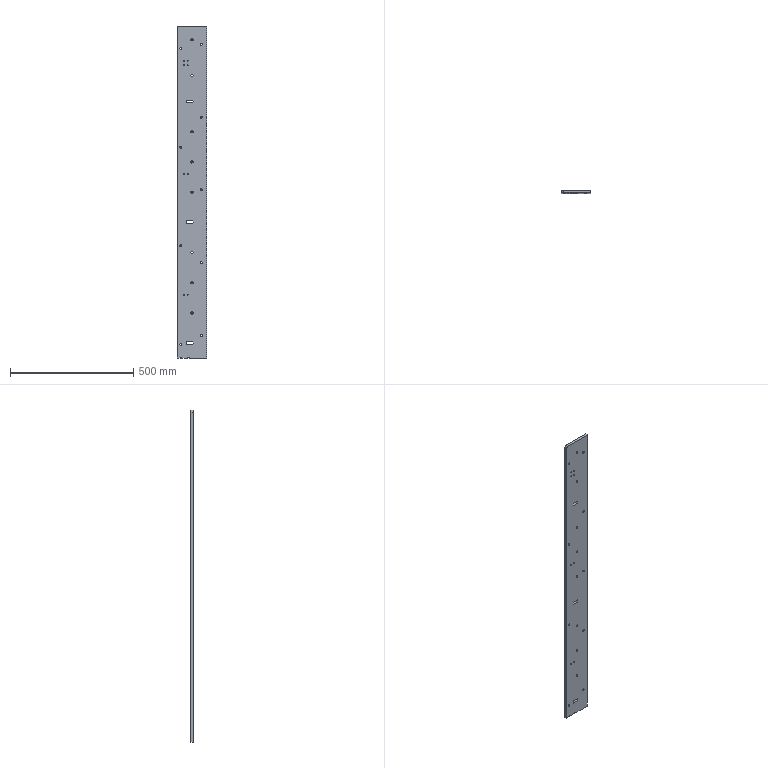Part | STEP file | 1 solid | 82 faces | box 120 x 10 x 1346 mm | volume 1594815 mm3 | cylinder 59 | plane 23 | commonest cylinder face diameters 4.2 x16 9 x16 8.4 x10 8.5 x8 2 x6 7 x2